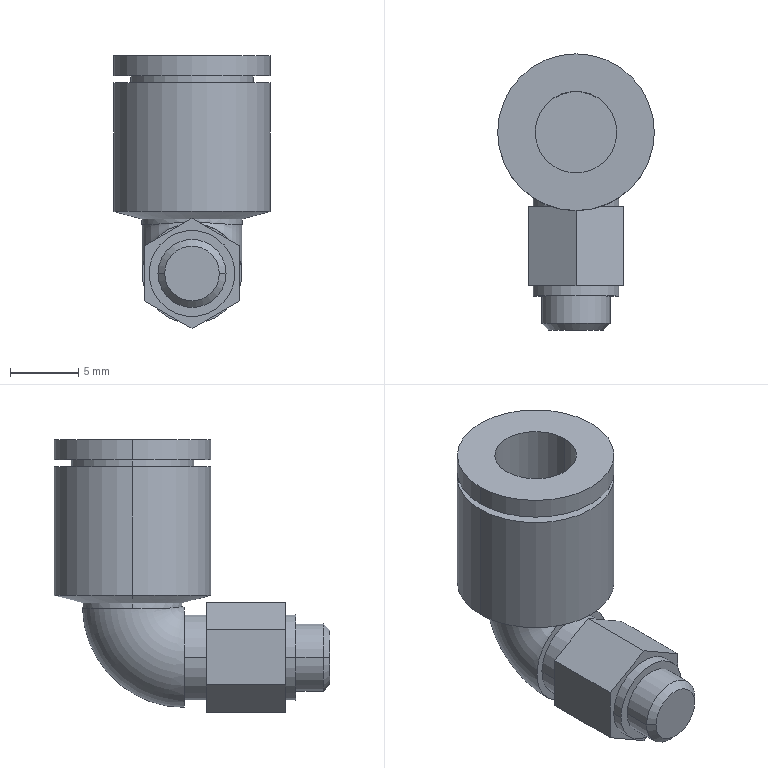Part | SolidWorks | features Revolution 3, ICE 2 | 1 solid | 38 faces | box 11.5 x 20.25 x 20.041 mm | volume 1442 mm3 | cylinder 16 | plane 16 | cone 4 | torus 2 | commonest cylinder face diameters 6.3 x4 11.5 x4 5 x2 6 x2 7.36 x2 9 x2
STEP:
#1=CARTESIAN_POINT('',(0.,18.166,3.565));
#2=VERTEX_POINT('',#1);
#3=CARTESIAN_POINT('',(-2.939,12.285,3.565));
#4=VERTEX_POINT('',#3);
#5=CARTESIAN_POINT('',(0.,18.166,3.565));
#6=CARTESIAN_POINT('',(-0.3422,18.166,3.565));
#7=CARTESIAN_POINT('',(-0.6763,18.119,3.565));
#8=CARTESIAN_POINT('',(-1.166,17.98,3.565));
#9=CARTESIAN_POINT('',(-1.328,17.922,3.565));
#10=CARTESIAN_POINT('',(-1.637,17.785,3.565));
#11=CARTESIAN_POINT('',(-1.787,17.706,3.565));
#12=CARTESIAN_POINT('',(-2.217,17.44,3.565));
#13=CARTESIAN_POINT('',(-2.484,17.219,3.565));
#14=CARTESIAN_POINT('',(-2.825,16.845,3.565));
#15=CARTESIAN_POINT('',(-2.93,16.713,3.565));
#16=CARTESIAN_POINT('',(-3.122,16.432,3.565));
#17=CARTESIAN_POINT('',(-3.209,16.284,3.565));
#18=CARTESIAN_POINT('',(-3.36,15.982,3.565));
#19=CARTESIAN_POINT('',(-3.424,15.826,3.565));
#20=CARTESIAN_POINT('',(-3.532,15.505,3.565));
#21=CARTESIAN_POINT('',(-3.575,15.339,3.565));
#22=CARTESIAN_POINT('',(-3.67,14.838,3.565));
#23=CARTESIAN_POINT('',(-3.686,14.501,3.565));
#24=CARTESIAN_POINT('',(-3.624,13.822,3.565));
#25=CARTESIAN_POINT('',(-3.547,13.491,3.565));
#26=CARTESIAN_POINT('',(-3.366,13.016,3.565));
#27=CARTESIAN_POINT('',(-3.294,12.86,3.565));
#28=CARTESIAN_POINT('',(-3.13,12.563,3.565));
#29=CARTESIAN_POINT('',(-3.039,12.421,3.565));
#30=CARTESIAN_POINT('',(-2.939,12.285,3.565));
#31=B_SPLINE_CURVE_WITH_KNOTS('',3,(#5,#6,#7,#8,#9,#10,#11,#12,#13,#14,#15,#16,#17,#18,#19,#20,#21,#22,#23,#24,#25,#26,#27,#28,#29,#30),.UNSPECIFIED.,.F.,.F.,(4,2,2,2,2,2,2,2,2,2,2,2,4),(0.,0.001012,0.001518,0.002024,0.003036,0.003542,0.004048,0.004554,0.00506,0.006072,0.007083,0.007589,0.008095),.UNSPECIFIED.);
#32=EDGE_CURVE('',#2,#4,#31,.T.);
#33=ORIENTED_EDGE('',*,*,#32,.F.);
#34=CARTESIAN_POINT('',(0.,10.705,-3.67));
#35=VERTEX_POINT('',#34);
#36=CARTESIAN_POINT('',(0.,10.705,3.795));
#37=DIRECTION('',(-1.,0.,0.));
#38=DIRECTION('',(0.,0.,1.));
#39=AXIS2_PLACEMENT_3D('',#36,#37,#38);
#40=CIRCLE('',#39,7.465);
#41=EDGE_CURVE('',#2,#35,#40,.T.);
#42=ORIENTED_EDGE('',*,*,#41,.T.);
#43=CARTESIAN_POINT('',(0.,10.705,3.67));
#44=VERTEX_POINT('',#43);
#45=CARTESIAN_POINT('',(0.,10.705,0.));
#46=DIRECTION('',(0.,1.,0.));
#47=DIRECTION('',(-1.,0.,0.));
#48=AXIS2_PLACEMENT_3D('',#45,#46,#47);
#49=CIRCLE('',#48,3.67);
#50=EDGE_CURVE('',#35,#44,#49,.T.);
#51=ORIENTED_EDGE('',*,*,#50,.T.);
#52=CARTESIAN_POINT('',(0.,10.82,3.746));
#53=VERTEX_POINT('',#52);
#54=CARTESIAN_POINT('',(0.,10.705,3.795));
#55=DIRECTION('',(-1.,0.,0.));
#56=DIRECTION('',(0.,0.,1.));
#57=AXIS2_PLACEMENT_3D('',#54,#55,#56);
#58=CIRCLE('',#57,0.125);
#59=EDGE_CURVE('',#53,#44,#58,.T.);
#60=ORIENTED_EDGE('',*,*,#59,.F.);
#61=CARTESIAN_POINT('',(-2.939,12.285,3.565));
#62=CARTESIAN_POINT('',(-2.767,12.057,3.593));
#63=CARTESIAN_POINT('',(-2.572,11.853,3.616));
#64=CARTESIAN_POINT('',(-2.137,11.491,3.656));
#65=CARTESIAN_POINT('',(-1.895,11.333,3.673));
#66=CARTESIAN_POINT('',(-1.389,11.081,3.704));
#67=CARTESIAN_POINT('',(-1.121,10.983,3.717));
#68=CARTESIAN_POINT('',(-0.5648,10.852,3.739));
#69=CARTESIAN_POINT('',(-0.2838,10.82,3.746));
#70=CARTESIAN_POINT('',(0.,10.82,3.746));
#71=B_SPLINE_CURVE_WITH_KNOTS('',3,(#61,#62,#63,#64,#65,#66,#67,#68,#69,#70),.UNSPECIFIED.,.F.,.F.,(4,2,2,2,4),(0.000001984,0.0008506,0.001699,0.002548,0.003397),.UNSPECIFIED.);
#72=EDGE_CURVE('',#4,#53,#71,.T.);
#73=ORIENTED_EDGE('',*,*,#72,.F.);
#74=EDGE_LOOP('',(#33,#42,#51,#60,#73));
#75=FACE_OUTER_BOUND('',#74,.T.);
#76=CARTESIAN_POINT('',(0.,10.705,3.795));
#77=DIRECTION('',(-1.,0.,0.));
#78=DIRECTION('',(0.,0.,1.));
#79=AXIS2_PLACEMENT_3D('',#76,#77,#78);
#80=TOROIDAL_SURFACE('',#79,3.795,3.67);
#81=ADVANCED_FACE('',(#75),#80,.T.);
#82=CARTESIAN_POINT('',(-3.,14.5,16.));
#83=VERTEX_POINT('',#82);
#84=CARTESIAN_POINT('',(3.,14.5,16.));
#85=VERTEX_POINT('',#84);
#86=CARTESIAN_POINT('',(0.,14.5,16.));
#87=DIRECTION('',(0.,0.,1.));
#88=DIRECTION('',(-1.,0.,0.));
#89=AXIS2_PLACEMENT_3D('',#86,#87,#88);
#90=CIRCLE('',#89,3.);
#91=EDGE_CURVE('',#83,#85,#90,.T.);
#92=ORIENTED_EDGE('',*,*,#91,.T.);
#93=CARTESIAN_POINT('',(3.,14.5,2.));
#94=VERTEX_POINT('',#93);
#95=CARTESIAN_POINT('',(3.,14.5,30.));
#96=DIRECTION('',(0.,0.,-1.));
#97=VECTOR('',#96,1000.);
#98=LINE('',#95,#97);
#99=EDGE_CURVE('',#85,#94,#98,.T.);
#100=ORIENTED_EDGE('',*,*,#99,.T.);
#101=CARTESIAN_POINT('',(-3.,14.5,2.));
#102=VERTEX_POINT('',#101);
#103=CARTESIAN_POINT('',(0.,14.5,2.));
#104=DIRECTION('',(0.,0.,1.));
#105=DIRECTION('',(1.,0.,0.));
#106=AXIS2_PLACEMENT_3D('',#103,#104,#105);
#107=CIRCLE('',#106,3.);
#108=EDGE_CURVE('',#102,#94,#107,.T.);
#109=ORIENTED_EDGE('',*,*,#108,.F.);
#110=CARTESIAN_POINT('',(-3.,14.5,30.));
#111=DIRECTION('',(0.,0.,-1.));
#112=VECTOR('',#111,1000.);
#113=LINE('',#110,#112);
#114=EDGE_CURVE('',#83,#102,#113,.T.);
#115=ORIENTED_EDGE('',*,*,#114,.F.);
#116=EDGE_LOOP('',(#92,#100,#109,#115));
#117=FACE_OUTER_BOUND('',#116,.T.);
#118=CARTESIAN_POINT('',(0.,14.5,30.));
#119=DIRECTION('',(0.,0.,-1.));
#120=DIRECTION('',(-1.,0.,0.));
#121=AXIS2_PLACEMENT_3D('',#118,#119,#120);
#122=CYLINDRICAL_SURFACE('',#121,3.);
#123=ADVANCED_FACE('',(#117),#122,.F.);
#124=CARTESIAN_POINT('',(3.68,14.5,4.));
#125=VERTEX_POINT('',#124);
#126=CARTESIAN_POINT('',(-3.68,14.5,4.));
#127=VERTEX_POINT('',#126);
#128=CARTESIAN_POINT('',(0.,14.5,4.));
#129=DIRECTION('',(0.,0.,1.));
#130=DIRECTION('',(1.,0.,0.));
#131=AXIS2_PLACEMENT_3D('',#128,#129,#130);
#132=CIRCLE('',#131,3.68);
#133=EDGE_CURVE('',#125,#127,#132,.T.);
#134=ORIENTED_EDGE('',*,*,#133,.T.);
#135=CARTESIAN_POINT('',(-5.75,14.5,4.555));
#136=VERTEX_POINT('',#135);
#137=CARTESIAN_POINT('',(-3.68,14.5,4.));
#138=DIRECTION('',(-0.9659,0.,0.2588));
#139=VECTOR('',#138,1000.);
#140=LINE('',#137,#139);
#141=EDGE_CURVE('',#127,#136,#140,.T.);
#142=ORIENTED_EDGE('',*,*,#141,.T.);
#143=CARTESIAN_POINT('',(5.75,14.5,4.555));
#144=VERTEX_POINT('',#143);
#145=CARTESIAN_POINT('',(0.,14.5,4.555));
#146=DIRECTION('',(0.,0.,1.));
#147=DIRECTION('',(1.,0.,0.));
#148=AXIS2_PLACEMENT_3D('',#145,#146,#147);
#149=CIRCLE('',#148,5.75);
#150=EDGE_CURVE('',#144,#136,#149,.T.);
#151=ORIENTED_EDGE('',*,*,#150,.F.);
#152=CARTESIAN_POINT('',(3.68,14.5,4.));
#153=DIRECTION('',(0.9659,0.,0.2588));
#154=VECTOR('',#153,1000.);
#155=LINE('',#152,#154);
#156=EDGE_CURVE('',#125,#144,#155,.T.);
#157=ORIENTED_EDGE('',*,*,#156,.F.);
#158=EDGE_LOOP('',(#134,#142,#151,#157));
#159=FACE_OUTER_BOUND('',#158,.T.);
#160=CARTESIAN_POINT('',(0.,14.5,4.));
#161=DIRECTION('',(0.,0.,1.));
#162=DIRECTION('',(1.,0.,0.));
#163=AXIS2_PLACEMENT_3D('',#160,#161,#162);
#164=CONICAL_SURFACE('',#163,3.68,1.309);
#165=ADVANCED_FACE('',(#159),#164,.T.);
#166=ORIENTED_EDGE('',*,*,#150,.T.);
#167=CARTESIAN_POINT('',(-5.75,14.5,14.));
#168=VERTEX_POINT('',#167);
#169=CARTESIAN_POINT('',(-5.75,14.5,3.565));
#170=DIRECTION('',(0.,0.,1.));
#171=VECTOR('',#170,1000.);
#172=LINE('',#169,#171);
#173=EDGE_CURVE('',#136,#168,#172,.T.);
#174=ORIENTED_EDGE('',*,*,#173,.T.);
#175=CARTESIAN_POINT('',(5.75,14.5,14.));
#176=VERTEX_POINT('',#175);
#177=CARTESIAN_POINT('',(0.,14.5,14.));
#178=DIRECTION('',(0.,0.,1.));
#179=DIRECTION('',(1.,0.,0.));
#180=AXIS2_PLACEMENT_3D('',#177,#178,#179);
#181=CIRCLE('',#180,5.75);
#182=EDGE_CURVE('',#176,#168,#181,.T.);
#183=ORIENTED_EDGE('',*,*,#182,.F.);
#184=CARTESIAN_POINT('',(5.75,14.5,3.565));
#185=DIRECTION('',(0.,0.,1.));
#186=VECTOR('',#185,1000.);
#187=LINE('',#184,#186);
#188=EDGE_CURVE('',#144,#176,#187,.T.);
#189=ORIENTED_EDGE('',*,*,#188,.F.);
#190=EDGE_LOOP('',(#166,#174,#183,#189));
#191=FACE_OUTER_BOUND('',#190,.T.);
#192=CARTESIAN_POINT('',(0.,14.5,3.565));
#193=DIRECTION('',(0.,0.,1.));
#194=DIRECTION('',(1.,0.,0.));
#195=AXIS2_PLACEMENT_3D('',#192,#193,#194);
#196=CYLINDRICAL_SURFACE('',#195,5.75);
#197=ADVANCED_FACE('',(#191),#196,.T.);
#198=CARTESIAN_POINT('',(4.5,14.5,14.));
#199=VERTEX_POINT('',#198);
#200=CARTESIAN_POINT('',(-4.5,14.5,14.));
#201=VERTEX_POINT('',#200);
#202=CARTESIAN_POINT('',(0.,14.5,14.));
#203=DIRECTION('',(0.,0.,1.));
#204=DIRECTION('',(1.,0.,0.));
#205=AXIS2_PLACEMENT_3D('',#202,#203,#204);
#206=CIRCLE('',#205,4.5);
#207=EDGE_CURVE('',#199,#201,#206,.T.);
#208=ORIENTED_EDGE('',*,*,#207,.T.);
#209=CARTESIAN_POINT('',(-4.5,14.5,14.5));
#210=VERTEX_POINT('',#209);
#211=CARTESIAN_POINT('',(-4.5,14.5,3.565));
#212=DIRECTION('',(0.,0.,1.));
#213=VECTOR('',#212,1000.);
#214=LINE('',#211,#213);
#215=EDGE_CURVE('',#201,#210,#214,.T.);
#216=ORIENTED_EDGE('',*,*,#215,.T.);
#217=CARTESIAN_POINT('',(4.5,14.5,14.5));
#218=VERTEX_POINT('',#217);
#219=CARTESIAN_POINT('',(0.,14.5,14.5));
#220=DIRECTION('',(0.,0.,1.));
#221=DIRECTION('',(1.,0.,0.));
#222=AXIS2_PLACEMENT_3D('',#219,#220,#221);
#223=CIRCLE('',#222,4.5);
#224=EDGE_CURVE('',#218,#210,#223,.T.);
#225=ORIENTED_EDGE('',*,*,#224,.F.);
#226=CARTESIAN_POINT('',(4.5,14.5,3.565));
#227=DIRECTION('',(0.,0.,1.));
#228=VECTOR('',#227,1000.);
#229=LINE('',#226,#228);
#230=EDGE_CURVE('',#199,#218,#229,.T.);
#231=ORIENTED_EDGE('',*,*,#230,.F.);
#232=EDGE_LOOP('',(#208,#216,#225,#231));
#233=FACE_OUTER_BOUND('',#232,.T.);
#234=CARTESIAN_POINT('',(0.,14.5,3.565));
#235=DIRECTION('',(0.,0.,1.));
#236=DIRECTION('',(1.,0.,0.));
#237=AXIS2_PLACEMENT_3D('',#234,#235,#236);
#238=CYLINDRICAL_SURFACE('',#237,4.5);
#239=ADVANCED_FACE('',(#233),#238,.T.);
#240=CARTESIAN_POINT('',(5.75,14.5,14.5));
#241=VERTEX_POINT('',#240);
#242=CARTESIAN_POINT('',(-5.75,14.5,14.5));
#243=VERTEX_POINT('',#242);
#244=CARTESIAN_POINT('',(0.,14.5,14.5));
#245=DIRECTION('',(0.,0.,1.));
#246=DIRECTION('',(1.,0.,0.));
#247=AXIS2_PLACEMENT_3D('',#244,#245,#246);
#248=CIRCLE('',#247,5.75);
#249=EDGE_CURVE('',#241,#243,#248,.T.);
#250=ORIENTED_EDGE('',*,*,#249,.T.);
#251=CARTESIAN_POINT('',(-5.75,14.5,16.));
#252=VERTEX_POINT('',#251);
#253=CARTESIAN_POINT('',(-5.75,14.5,3.565));
#254=DIRECTION('',(0.,0.,1.));
#255=VECTOR('',#254,1000.);
#256=LINE('',#253,#255);
#257=EDGE_CURVE('',#243,#252,#256,.T.);
#258=ORIENTED_EDGE('',*,*,#257,.T.);
#259=CARTESIAN_POINT('',(5.75,14.5,16.));
#260=VERTEX_POINT('',#259);
#261=CARTESIAN_POINT('',(0.,14.5,16.));
#262=DIRECTION('',(0.,0.,1.));
#263=DIRECTION('',(1.,0.,0.));
#264=AXIS2_PLACEMENT_3D('',#261,#262,#263);
#265=CIRCLE('',#264,5.75);
#266=EDGE_CURVE('',#260,#252,#265,.T.);
#267=ORIENTED_EDGE('',*,*,#266,.F.);
#268=CARTESIAN_POINT('',(5.75,14.5,3.565));
#269=DIRECTION('',(0.,0.,1.));
#270=VECTOR('',#269,1000.);
#271=LINE('',#268,#270);
#272=EDGE_CURVE('',#241,#260,#271,.T.);
#273=ORIENTED_EDGE('',*,*,#272,.F.);
#274=EDGE_LOOP('',(#250,#258,#267,#273));
#275=FACE_OUTER_BOUND('',#274,.T.);
#276=CARTESIAN_POINT('',(0.,14.5,3.565));
#277=DIRECTION('',(0.,0.,1.));
#278=DIRECTION('',(1.,0.,0.));
#279=AXIS2_PLACEMENT_3D('',#276,#277,#278);
#280=CYLINDRICAL_SURFACE('',#279,5.75);
#281=ADVANCED_FACE('',(#275),#280,.T.);
#282=CARTESIAN_POINT('',(3.68,14.5,3.565));
#283=VERTEX_POINT('',#282);
#284=CARTESIAN_POINT('',(-3.68,14.5,3.565));
#285=VERTEX_POINT('',#284);
#286=CARTESIAN_POINT('',(0.,14.5,3.565));
#287=DIRECTION('',(0.,0.,1.));
#288=DIRECTION('',(1.,0.,0.));
#289=AXIS2_PLACEMENT_3D('',#286,#287,#288);
#290=CIRCLE('',#289,3.68);
#291=EDGE_CURVE('',#283,#285,#290,.T.);
#292=ORIENTED_EDGE('',*,*,#291,.T.);
#293=CARTESIAN_POINT('',(-3.68,14.5,3.565));
#294=DIRECTION('',(0.,0.,1.));
#295=VECTOR('',#294,1000.);
#296=LINE('',#293,#295);
#297=EDGE_CURVE('',#285,#127,#296,.T.);
#298=ORIENTED_EDGE('',*,*,#297,.T.);
#299=ORIENTED_EDGE('',*,*,#133,.F.);
#300=CARTESIAN_POINT('',(3.68,14.5,3.565));
#301=DIRECTION('',(0.,0.,1.));
#302=VECTOR('',#301,1000.);
#303=LINE('',#300,#302);
#304=EDGE_CURVE('',#283,#125,#303,.T.);
#305=ORIENTED_EDGE('',*,*,#304,.F.);
#306=EDGE_LOOP('',(#292,#298,#299,#305));
#307=FACE_OUTER_BOUND('',#306,.T.);
#308=CARTESIAN_POINT('',(0.,14.5,3.565));
#309=DIRECTION('',(0.,0.,1.));
#310=DIRECTION('',(1.,0.,0.));
#311=AXIS2_PLACEMENT_3D('',#308,#309,#310);
#312=CYLINDRICAL_SURFACE('',#311,3.68);
#313=ADVANCED_FACE('',(#307),#312,.T.);
#314=CARTESIAN_POINT('',(-3.15,10.705,0.));
#315=VERTEX_POINT('',#314);
#316=CARTESIAN_POINT('',(3.15,10.705,0.));
#317=VERTEX_POINT('',#316);
#318=CARTESIAN_POINT('',(0.,10.705,0.));
#319=DIRECTION('',(0.,1.,0.));
#320=DIRECTION('',(-1.,0.,0.));
#321=AXIS2_PLACEMENT_3D('',#318,#319,#320);
#322=CIRCLE('',#321,3.15);
#323=EDGE_CURVE('',#315,#317,#322,.T.);
#324=ORIENTED_EDGE('',*,*,#323,.F.);
#325=CARTESIAN_POINT('',(-3.15,9.05,0.));
#326=VERTEX_POINT('',#325);
#327=CARTESIAN_POINT('',(-3.15,10.705,0.));
#328=DIRECTION('',(0.,-1.,0.));
#329=VECTOR('',#328,1000.);
#330=LINE('',#327,#329);
#331=EDGE_CURVE('',#315,#326,#330,.T.);
#332=ORIENTED_EDGE('',*,*,#331,.T.);
#333=CARTESIAN_POINT('',(3.15,9.05,0.));
#334=VERTEX_POINT('',#333);
#335=CARTESIAN_POINT('',(0.,9.05,0.));
#336=DIRECTION('',(0.,1.,0.));
#337=DIRECTION('',(0.,0.,1.));
#338=AXIS2_PLACEMENT_3D('',#335,#336,#337);
#339=CIRCLE('',#338,3.15);
#340=EDGE_CURVE('',#326,#334,#339,.T.);
#341=ORIENTED_EDGE('',*,*,#340,.T.);
#342=CARTESIAN_POINT('',(3.15,10.705,0.));
#343=DIRECTION('',(0.,-1.,0.));
#344=VECTOR('',#343,1000.);
#345=LINE('',#342,#344);
#346=EDGE_CURVE('',#317,#334,#345,.T.);
#347=ORIENTED_EDGE('',*,*,#346,.F.);
#348=EDGE_LOOP('',(#324,#332,#341,#347));
#349=FACE_OUTER_BOUND('',#348,.T.);
#350=CARTESIAN_POINT('',(0.,10.705,0.));
#351=DIRECTION('',(0.,-1.,0.));
#352=DIRECTION('',(1.,0.,0.));
#353=AXIS2_PLACEMENT_3D('',#350,#351,#352);
#354=CYLINDRICAL_SURFACE('',#353,3.15);
#355=ADVANCED_FACE('',(#349),#354,.T.);
#356=CARTESIAN_POINT('',(2.5,2.5,0.));
#357=VERTEX_POINT('',#356);
#358=CARTESIAN_POINT('',(-2.5,2.5,0.));
#359=VERTEX_POINT('',#358);
#360=CARTESIAN_POINT('',(0.,2.5,0.));
#361=DIRECTION('',(0.,-1.,0.));
#362=DIRECTION('',(1.,0.,0.));
#363=AXIS2_PLACEMENT_3D('',#360,#361,#362);
#364=CIRCLE('',#363,2.5);
#365=EDGE_CURVE('',#357,#359,#364,.T.);
#366=ORIENTED_EDGE('',*,*,#365,.T.);
#367=CARTESIAN_POINT('',(-2.5,0.49,0.));
#368=VERTEX_POINT('',#367);
#369=CARTESIAN_POINT('',(-2.5,10.705,0.));
#370=DIRECTION('',(0.,-1.,0.));
#371=VECTOR('',#370,1000.);
#372=LINE('',#369,#371);
#373=EDGE_CURVE('',#359,#368,#372,.T.);
#374=ORIENTED_EDGE('',*,*,#373,.T.);
#375=CARTESIAN_POINT('',(2.5,0.49,0.));
#376=VERTEX_POINT('',#375);
#377=CARTESIAN_POINT('',(0.,0.49,0.));
#378=DIRECTION('',(0.,-1.,0.));
#379=DIRECTION('',(1.,0.,0.));
#380=AXIS2_PLACEMENT_3D('',#377,#378,#379);
#381=CIRCLE('',#380,2.5);
#382=EDGE_CURVE('',#376,#368,#381,.T.);
#383=ORIENTED_EDGE('',*,*,#382,.F.);
#384=CARTESIAN_POINT('',(2.5,10.705,0.));
#385=DIRECTION('',(0.,-1.,0.));
#386=VECTOR('',#385,1000.);
#387=LINE('',#384,#386);
#388=EDGE_CURVE('',#357,#376,#387,.T.);
#389=ORIENTED_EDGE('',*,*,#388,.F.);
#390=EDGE_LOOP('',(#366,#374,#383,#389));
#391=FACE_OUTER_BOUND('',#390,.T.);
#392=CARTESIAN_POINT('',(0.,10.705,0.));
#393=DIRECTION('',(0.,-1.,0.));
#394=DIRECTION('',(1.,0.,0.));
#395=AXIS2_PLACEMENT_3D('',#392,#393,#394);
#396=CYLINDRICAL_SURFACE('',#395,2.5);
#397=ADVANCED_FACE('',(#391),#396,.T.);
#398=CARTESIAN_POINT('',(2.01,0.,0.));
#399=VERTEX_POINT('',#398);
#400=CARTESIAN_POINT('',(-2.01,0.,0.));
#401=VERTEX_POINT('',#400);
#402=CARTESIAN_POINT('',(0.,0.,0.));
#403=DIRECTION('',(0.,-1.,0.));
#404=DIRECTION('',(1.,0.,0.));
#405=AXIS2_PLACEMENT_3D('',#402,#403,#404);
#406=CIRCLE('',#405,2.01);
#407=EDGE_CURVE('',#399,#401,#406,.T.);
#408=ORIENTED_EDGE('',*,*,#407,.F.);
#409=CARTESIAN_POINT('',(2.5,0.49,0.));
#410=DIRECTION('',(0.7071,0.7071,0.));
#411=VECTOR('',#410,1000.);
#412=LINE('',#409,#411);
#413=EDGE_CURVE('',#399,#376,#412,.T.);
#414=ORIENTED_EDGE('',*,*,#413,.T.);
#415=ORIENTED_EDGE('',*,*,#382,.T.);
#416=CARTESIAN_POINT('',(-2.5,0.49,0.));
#417=DIRECTION('',(-0.7071,0.7071,0.));
#418=VECTOR('',#417,1000.);
#419=LINE('',#416,#418);
#420=EDGE_CURVE('',#401,#368,#419,.T.);
#421=ORIENTED_EDGE('',*,*,#420,.F.);
#422=EDGE_LOOP('',(#408,#414,#415,#421));
#423=FACE_OUTER_BOUND('',#422,.T.);
#424=CARTESIAN_POINT('',(0.,0.49,0.));
#425=DIRECTION('',(0.,1.,0.));
#426=DIRECTION('',(-1.,0.,0.));
#427=AXIS2_PLACEMENT_3D('',#424,#425,#426);
#428=CONICAL_SURFACE('',#427,2.5,0.7854);
#429=ADVANCED_FACE('',(#423),#428,.T.);
#430=CARTESIAN_POINT('',(-3.15,3.25,0.));
#431=VERTEX_POINT('',#430);
#432=CARTESIAN_POINT('',(3.15,3.25,0.));
#433=VERTEX_POINT('',#432);
#434=CARTESIAN_POINT('',(0.,3.25,0.));
#435=DIRECTION('',(0.,1.,0.));
#436=DIRECTION('',(0.,0.,1.));
#437=AXIS2_PLACEMENT_3D('',#434,#435,#436);
#438=CIRCLE('',#437,3.15);
#439=EDGE_CURVE('',#431,#433,#438,.T.);
#440=ORIENTED_EDGE('',*,*,#439,.F.);
#441=CARTESIAN_POINT('',(-3.15,2.5,0.));
#442=VERTEX_POINT('',#441);
#443=CARTESIAN_POINT('',(-3.15,10.705,0.));
#444=DIRECTION('',(0.,-1.,0.));
#445=VECTOR('',#444,1000.);
#446=LINE('',#443,#445);
#447=EDGE_CURVE('',#431,#442,#446,.T.);
#448=ORIENTED_EDGE('',*,*,#447,.T.);
#449=CARTESIAN_POINT('',(3.15,2.5,0.));
#450=VERTEX_POINT('',#449);
#451=CARTESIAN_POINT('',(0.,2.5,0.));
#452=DIRECTION('',(0.,-1.,0.));
#453=DIRECTION('',(1.,0.,0.));
#454=AXIS2_PLACEMENT_3D('',#451,#452,#453);
#455=CIRCLE('',#454,3.15);
#456=EDGE_CURVE('',#450,#442,#455,.T.);
#457=ORIENTED_EDGE('',*,*,#456,.F.);
#458=CARTESIAN_POINT('',(3.15,10.705,0.));
#459=DIRECTION('',(0.,-1.,0.));
#460=VECTOR('',#459,1000.);
#461=LINE('',#458,#460);
#462=EDGE_CURVE('',#433,#450,#461,.T.);
#463=ORIENTED_EDGE('',*,*,#462,.F.);
#464=EDGE_LOOP('',(#440,#448,#457,#463));
#465=FACE_OUTER_BOUND('',#464,.T.);
#466=CARTESIAN_POINT('',(0.,10.705,0.));
#467=DIRECTION('',(0.,-1.,0.));
#468=DIRECTION('',(1.,0.,0.));
#469=AXIS2_PLACEMENT_3D('',#466,#467,#468);
#470=CYLINDRICAL_SURFACE('',#469,3.15);
#471=ADVANCED_FACE('',(#465),#470,.T.);
#472=ORIENTED_EDGE('',*,*,#266,.T.);
#473=CARTESIAN_POINT('',(0.,14.5,16.));
#474=DIRECTION('',(0.,0.,1.));
#475=DIRECTION('',(1.,0.,0.));
#476=AXIS2_PLACEMENT_3D('',#473,#474,#475);
#477=CIRCLE('',#476,5.75);
#478=EDGE_CURVE('',#252,#260,#477,.T.);
#479=ORIENTED_EDGE('',*,*,#478,.T.);
#480=EDGE_LOOP('',(#472,#479));
#481=FACE_OUTER_BOUND('',#480,.T.);
#482=ORIENTED_EDGE('',*,*,#91,.F.);
#483=CARTESIAN_POINT('',(0.,14.5,16.));
#484=DIRECTION('',(0.,0.,1.));
#485=DIRECTION('',(-1.,0.,0.));
#486=AXIS2_PLACEMENT_3D('',#483,#484,#485);
#487=CIRCLE('',#486,3.);
#488=EDGE_CURVE('',#85,#83,#487,.T.);
#489=ORIENTED_EDGE('',*,*,#488,.F.);
#490=EDGE_LOOP('',(#482,#489));
#491=FACE_BOUND('',#490,.T.);
#492=CARTESIAN_POINT('',(0.,14.5,16.));
#493=DIRECTION('',(0.,0.,-1.));
#494=DIRECTION('',(-1.,0.,0.));
#495=AXIS2_PLACEMENT_3D('',#492,#493,#494);
#496=PLANE('',#495);
#497=ADVANCED_FACE('',(#481,#491),#496,.F.);
#498=ORIENTED_EDGE('',*,*,#41,.F.);
#499=CARTESIAN_POINT('',(2.939,12.285,3.565));
#500=VERTEX_POINT('',#499);
#501=CARTESIAN_POINT('',(2.939,12.285,3.565));
#502=CARTESIAN_POINT('',(3.04,12.422,3.565));
#503=CARTESIAN_POINT('',(3.132,12.566,3.565));
#504=CARTESIAN_POINT('',(3.294,12.862,3.565));
#505=CARTESIAN_POINT('',(3.365,13.014,3.565));
#506=CARTESIAN_POINT('',(3.486,13.329,3.565));
#507=CARTESIAN_POINT('',(3.536,13.493,3.565));
#508=CARTESIAN_POINT('',(3.613,13.825,3.565));
#509=CARTESIAN_POINT('',(3.666,14.158,3.565));
#510=CARTESIAN_POINT('',(3.674,14.496,3.565));
#511=CARTESIAN_POINT('',(3.658,14.836,3.565));
#512=CARTESIAN_POINT('',(3.638,15.006,3.565));
#513=CARTESIAN_POINT('',(3.576,15.338,3.565));
#514=CARTESIAN_POINT('',(3.533,15.501,3.565));
#515=CARTESIAN_POINT('',(3.426,15.822,3.565));
#516=CARTESIAN_POINT('',(3.36,15.98,3.565));
#517=CARTESIAN_POINT('',(3.133,16.437,3.565));
#518=CARTESIAN_POINT('',(2.943,16.715,3.565));
#519=CARTESIAN_POINT('',(2.484,17.219,3.565));
#520=CARTESIAN_POINT('',(2.222,17.436,3.565));
#521=CARTESIAN_POINT('',(1.791,17.704,3.565));
#522=CARTESIAN_POINT('',(1.639,17.784,3.565));
#523=CARTESIAN_POINT('',(1.328,17.922,3.565));
#524=CARTESIAN_POINT('',(1.17,17.979,3.565));
#525=CARTESIAN_POINT('',(0.8455,18.072,3.565));
#526=CARTESIAN_POINT('',(0.6799,18.107,3.565));
#527=CARTESIAN_POINT('',(0.4261,18.143,3.565));
#528=CARTESIAN_POINT('',(0.341,18.152,3.565));
#529=CARTESIAN_POINT('',(0.1708,18.163,3.565));
#530=CARTESIAN_POINT('',(0.08395,18.166,3.565));
#531=CARTESIAN_POINT('',(0.,18.166,3.565));
#532=B_SPLINE_CURVE_WITH_KNOTS('',3,(#501,#502,#503,#504,#505,#506,#507,#508,#509,#510,#511,#512,#513,#514,#515,#516,#517,#518,#519,#520,#521,#522,#523,#524,#525,#526,#527,#528,#529,#530,#531),.UNSPECIFIED.,.F.,.F.,(4,2,2,2,1,2,2,2,2,2,2,2,2,2,2,4),(0.03478,0.03528,0.03578,0.03627,0.03677,0.03727,0.03776,0.03826,0.03876,0.03975,0.04074,0.04124,0.04174,0.04223,0.04248,0.04273),.UNSPECIFIED.);
#533=EDGE_CURVE('',#500,#2,#532,.T.);
#534=ORIENTED_EDGE('',*,*,#533,.F.);
#535=CARTESIAN_POINT('',(0.,10.82,3.746));
#536=CARTESIAN_POINT('',(0.2832,10.82,3.746));
#537=CARTESIAN_POINT('',(0.5699,10.853,3.739));
#538=CARTESIAN_POINT('',(1.119,10.983,3.717));
#539=CARTESIAN_POINT('',(1.389,11.08,3.704));
#540=CARTESIAN_POINT('',(1.897,11.334,3.673));
#541=CARTESIAN_POINT('',(2.133,11.488,3.656));
#542=CARTESIAN_POINT('',(2.569,11.85,3.616));
#543=CARTESIAN_POINT('',(2.767,12.057,3.593));
#544=CARTESIAN_POINT('',(2.939,12.285,3.565));
#545=B_SPLINE_CURVE_WITH_KNOTS('',3,(#535,#536,#537,#538,#539,#540,#541,#542,#543,#544),.UNSPECIFIED.,.F.,.F.,(4,2,2,2,4),(0.003397,0.004243,0.00509,0.005937,0.006784),.UNSPECIFIED.);
#546=EDGE_CURVE('',#53,#500,#545,.T.);
#547=ORIENTED_EDGE('',*,*,#546,.F.);
#548=ORIENTED_EDGE('',*,*,#59,.T.);
#549=CARTESIAN_POINT('',(0.,10.705,0.));
#550=DIRECTION('',(0.,1.,0.));
#551=DIRECTION('',(-1.,0.,0.));
#552=AXIS2_PLACEMENT_3D('',#549,#550,#551);
#553=CIRCLE('',#552,3.67);
#554=EDGE_CURVE('',#44,#35,#553,.T.);
#555=ORIENTED_EDGE('',*,*,#554,.T.);
#556=EDGE_LOOP('',(#498,#534,#547,#548,#555));
#557=FACE_OUTER_BOUND('',#556,.T.);
#558=CARTESIAN_POINT('',(0.,10.705,3.795));
#559=DIRECTION('',(-1.,0.,0.));
#560=DIRECTION('',(0.,0.,1.));
#561=AXIS2_PLACEMENT_3D('',#558,#559,#560);
#562=TOROIDAL_SURFACE('',#561,3.795,3.67);
#563=ADVANCED_FACE('',(#557),#562,.T.);
#564=ORIENTED_EDGE('',*,*,#447,.F.);
#565=CARTESIAN_POINT('',(0.,3.25,0.));
#566=DIRECTION('',(0.,1.,0.));
#567=DIRECTION('',(0.,0.,1.));
#568=AXIS2_PLACEMENT_3D('',#565,#566,#567);
#569=CIRCLE('',#568,3.15);
#570=EDGE_CURVE('',#433,#431,#569,.T.);
#571=ORIENTED_EDGE('',*,*,#570,.F.);
#572=ORIENTED_EDGE('',*,*,#462,.T.);
#573=CARTESIAN_POINT('',(0.,2.5,0.));
#574=DIRECTION('',(0.,-1.,0.));
#575=DIRECTION('',(1.,0.,0.));
#576=AXIS2_PLACEMENT_3D('',#573,#574,#575);
#577=CIRCLE('',#576,3.15);
#578=EDGE_CURVE('',#442,#450,#577,.T.);
#579=ORIENTED_EDGE('',*,*,#578,.F.);
#580=EDGE_LOOP('',(#564,#571,#572,#579));
#581=FACE_OUTER_BOUND('',#580,.T.);
#582=CARTESIAN_POINT('',(0.,10.705,0.));
#583=DIRECTION('',(0.,-1.,0.));
#584=DIRECTION('',(1.,0.,0.));
#585=AXIS2_PLACEMENT_3D('',#582,#583,#584);
#586=CYLINDRICAL_SURFACE('',#585,3.15);
#587=ADVANCED_FACE('',(#581),#586,.T.);
#588=CARTESIAN_POINT('',(0.,0.,0.));
#589=DIRECTION('',(0.,-1.,0.));
#590=DIRECTION('',(1.,0.,0.));
#591=AXIS2_PLACEMENT_3D('',#588,#589,#590);
#592=CIRCLE('',#591,2.01);
#593=EDGE_CURVE('',#401,#399,#592,.T.);
#594=ORIENTED_EDGE('',*,*,#593,.T.);
#595=ORIENTED_EDGE('',*,*,#407,.T.);
#596=EDGE_LOOP('',(#594,#595));
#597=FACE_OUTER_BOUND('',#596,.T.);
#598=CARTESIAN_POINT('',(0.,0.,0.));
#599=DIRECTION('',(0.,1.,0.));
#600=DIRECTION('',(-1.,0.,0.));
#601=AXIS2_PLACEMENT_3D('',#598,#599,#600);
#602=PLANE('',#601);
#603=ADVANCED_FACE('',(#597),#602,.F.);
#604=ORIENTED_EDGE('',*,*,#413,.F.);
#605=ORIENTED_EDGE('',*,*,#593,.F.);
#606=ORIENTED_EDGE('',*,*,#420,.T.);
#607=CARTESIAN_POINT('',(0.,0.49,0.));
#608=DIRECTION('',(0.,-1.,0.));
#609=DIRECTION('',(1.,0.,0.));
#610=AXIS2_PLACEMENT_3D('',#607,#608,#609);
#611=CIRCLE('',#610,2.5);
#612=EDGE_CURVE('',#368,#376,#611,.T.);
#613=ORIENTED_EDGE('',*,*,#612,.T.);
#614=EDGE_LOOP('',(#604,#605,#606,#613));
#615=FACE_OUTER_BOUND('',#614,.T.);
#616=CARTESIAN_POINT('',(0.,0.49,0.));
#617=DIRECTION('',(0.,1.,0.));
#618=DIRECTION('',(-1.,0.,0.));
#619=AXIS2_PLACEMENT_3D('',#616,#617,#618);
#620=CONICAL_SURFACE('',#619,2.5,0.7854);
#621=ADVANCED_FACE('',(#615),#620,.T.);
#622=ORIENTED_EDGE('',*,*,#373,.F.);
#623=CARTESIAN_POINT('',(0.,2.5,0.));
#624=DIRECTION('',(0.,-1.,0.));
#625=DIRECTION('',(1.,0.,0.));
#626=AXIS2_PLACEMENT_3D('',#623,#624,#625);
#627=CIRCLE('',#626,2.5);
#628=EDGE_CURVE('',#359,#357,#627,.T.);
#629=ORIENTED_EDGE('',*,*,#628,.T.);
#630=ORIENTED_EDGE('',*,*,#388,.T.);
#631=ORIENTED_EDGE('',*,*,#612,.F.);
#632=EDGE_LOOP('',(#622,#629,#630,#631));
#633=FACE_OUTER_BOUND('',#632,.T.);
#634=CARTESIAN_POINT('',(0.,10.705,0.));
#635=DIRECTION('',(0.,-1.,0.));
#636=DIRECTION('',(1.,0.,0.));
#637=AXIS2_PLACEMENT_3D('',#634,#635,#636);
#638=CYLINDRICAL_SURFACE('',#637,2.5);
#639=ADVANCED_FACE('',(#633),#638,.T.);
#640=ORIENTED_EDGE('',*,*,#365,.F.);
#641=ORIENTED_EDGE('',*,*,#628,.F.);
#642=EDGE_LOOP('',(#640,#641));
#643=FACE_BOUND('',#642,.T.);
#644=ORIENTED_EDGE('',*,*,#456,.T.);
#645=ORIENTED_EDGE('',*,*,#578,.T.);
#646=EDGE_LOOP('',(#644,#645));
#647=FACE_OUTER_BOUND('',#646,.T.);
#648=CARTESIAN_POINT('',(-2.5,2.5,0.));
#649=DIRECTION('',(0.,1.,0.));
#650=DIRECTION('',(-1.,0.,0.));
#651=AXIS2_PLACEMENT_3D('',#648,#649,#650);
#652=PLANE('',#651);
#653=ADVANCED_FACE('',(#643,#647),#652,.F.);
#654=CARTESIAN_POINT('',(0.,9.05,-4.041));
#655=VERTEX_POINT('',#654);
#656=CARTESIAN_POINT('',(-3.5,9.05,-2.021));
#657=VERTEX_POINT('',#656);
#658=CARTESIAN_POINT('',(0.,9.05,-4.041));
#659=DIRECTION('',(-0.866,0.,0.5));
#660=VECTOR('',#659,1000.);
#661=LINE('',#658,#660);
#662=EDGE_CURVE('',#655,#657,#661,.T.);
#663=ORIENTED_EDGE('',*,*,#662,.T.);
#664=CARTESIAN_POINT('',(-3.5,9.05,2.021));
#665=VERTEX_POINT('',#664);
#666=CARTESIAN_POINT('',(-3.5,9.05,-2.021));
#667=DIRECTION('',(0.,0.,1.));
#668=VECTOR('',#667,1000.);
#669=LINE('',#666,#668);
#670=EDGE_CURVE('',#657,#665,#669,.T.);
#671=ORIENTED_EDGE('',*,*,#670,.T.);
#672=CARTESIAN_POINT('',(0.,9.05,4.041));
#673=VERTEX_POINT('',#672);
#674=CARTESIAN_POINT('',(-3.5,9.05,2.021));
#675=DIRECTION('',(0.866,0.,0.5));
#676=VECTOR('',#675,1000.);
#677=LINE('',#674,#676);
#678=EDGE_CURVE('',#665,#673,#677,.T.);
#679=ORIENTED_EDGE('',*,*,#678,.T.);
#680=CARTESIAN_POINT('',(3.5,9.05,2.021));
#681=VERTEX_POINT('',#680);
#682=CARTESIAN_POINT('',(0.,9.05,4.041));
#683=DIRECTION('',(0.866,0.,-0.5));
#684=VECTOR('',#683,1000.);
#685=LINE('',#682,#684);
#686=EDGE_CURVE('',#673,#681,#685,.T.);
#687=ORIENTED_EDGE('',*,*,#686,.T.);
#688=CARTESIAN_POINT('',(3.5,9.05,-2.021));
#689=VERTEX_POINT('',#688);
#690=CARTESIAN_POINT('',(3.5,9.05,2.021));
#691=DIRECTION('',(0.,0.,-1.));
#692=VECTOR('',#691,1000.);
#693=LINE('',#690,#692);
#694=EDGE_CURVE('',#681,#689,#693,.T.);
#695=ORIENTED_EDGE('',*,*,#694,.T.);
#696=CARTESIAN_POINT('',(3.5,9.05,-2.021));
#697=DIRECTION('',(-0.866,0.,-0.5));
#698=VECTOR('',#697,1000.);
#699=LINE('',#696,#698);
#700=EDGE_CURVE('',#689,#655,#699,.T.);
#701=ORIENTED_EDGE('',*,*,#700,.T.);
#702=EDGE_LOOP('',(#663,#671,#679,#687,#695,#701));
#703=FACE_OUTER_BOUND('',#702,.T.);
#704=CARTESIAN_POINT('',(0.,9.05,0.));
#705=DIRECTION('',(0.,1.,0.));
#706=DIRECTION('',(0.,0.,1.));
#707=AXIS2_PLACEMENT_3D('',#704,#705,#706);
#708=CIRCLE('',#707,3.15);
#709=EDGE_CURVE('',#334,#326,#708,.T.);
#710=ORIENTED_EDGE('',*,*,#709,.F.);
#711=ORIENTED_EDGE('',*,*,#340,.F.);
#712=EDGE_LOOP('',(#710,#711));
#713=FACE_BOUND('',#712,.T.);
#714=CARTESIAN_POINT('',(0.,9.05,0.));
#715=DIRECTION('',(0.,1.,0.));
#716=DIRECTION('',(0.,0.,1.));
#717=AXIS2_PLACEMENT_3D('',#714,#715,#716);
#718=PLANE('',#717);
#719=ADVANCED_FACE('',(#703,#713),#718,.T.);
#720=CARTESIAN_POINT('',(0.,3.25,-4.041));
#721=VERTEX_POINT('',#720);
#722=CARTESIAN_POINT('',(-3.5,3.25,-2.021));
#723=VERTEX_POINT('',#722);
#724=CARTESIAN_POINT('',(0.,3.25,-4.041));
#725=DIRECTION('',(-0.866,0.,0.5));
#726=VECTOR('',#725,1000.);
#727=LINE('',#724,#726);
#728=EDGE_CURVE('',#721,#723,#727,.T.);
#729=ORIENTED_EDGE('',*,*,#728,.F.);
#730=CARTESIAN_POINT('',(3.5,3.25,-2.021));
#731=VERTEX_POINT('',#730);
#732=CARTESIAN_POINT('',(3.5,3.25,-2.021));
#733=DIRECTION('',(-0.866,0.,-0.5));
#734=VECTOR('',#733,1000.);
#735=LINE('',#732,#734);
#736=EDGE_CURVE('',#731,#721,#735,.T.);
#737=ORIENTED_EDGE('',*,*,#736,.F.);
#738=CARTESIAN_POINT('',(3.5,3.25,2.021));
#739=VERTEX_POINT('',#738);
#740=CARTESIAN_POINT('',(3.5,3.25,2.021));
#741=DIRECTION('',(0.,0.,-1.));
#742=VECTOR('',#741,1000.);
#743=LINE('',#740,#742);
#744=EDGE_CURVE('',#739,#731,#743,.T.);
#745=ORIENTED_EDGE('',*,*,#744,.F.);
#746=CARTESIAN_POINT('',(0.,3.25,4.041));
#747=VERTEX_POINT('',#746);
#748=CARTESIAN_POINT('',(0.,3.25,4.041));
#749=DIRECTION('',(0.866,0.,-0.5));
#750=VECTOR('',#749,1000.);
#751=LINE('',#748,#750);
#752=EDGE_CURVE('',#747,#739,#751,.T.);
#753=ORIENTED_EDGE('',*,*,#752,.F.);
#754=CARTESIAN_POINT('',(-3.5,3.25,2.021));
#755=VERTEX_POINT('',#754);
#756=CARTESIAN_POINT('',(-3.5,3.25,2.021));
#757=DIRECTION('',(0.866,0.,0.5));
#758=VECTOR('',#757,1000.);
#759=LINE('',#756,#758);
#760=EDGE_CURVE('',#755,#747,#759,.T.);
#761=ORIENTED_EDGE('',*,*,#760,.F.);
#762=CARTESIAN_POINT('',(-3.5,3.25,-2.021));
#763=DIRECTION('',(0.,0.,1.));
#764=VECTOR('',#763,1000.);
#765=LINE('',#762,#764);
#766=EDGE_CURVE('',#723,#755,#765,.T.);
#767=ORIENTED_EDGE('',*,*,#766,.F.);
#768=EDGE_LOOP('',(#729,#737,#745,#753,#761,#767));
#769=FACE_OUTER_BOUND('',#768,.T.);
#770=ORIENTED_EDGE('',*,*,#570,.T.);
#771=ORIENTED_EDGE('',*,*,#439,.T.);
#772=EDGE_LOOP('',(#770,#771));
#773=FACE_BOUND('',#772,.T.);
#774=CARTESIAN_POINT('',(0.,3.25,0.));
#775=DIRECTION('',(0.,1.,0.));
#776=DIRECTION('',(0.,0.,1.));
#777=AXIS2_PLACEMENT_3D('',#774,#775,#776);
#778=PLANE('',#777);
#779=ADVANCED_FACE('',(#769,#773),#778,.F.);
#780=ORIENTED_EDGE('',*,*,#728,.T.);
#781=CARTESIAN_POINT('',(-3.5,9.05,-2.021));
#782=DIRECTION('',(0.,-1.,0.));
#783=VECTOR('',#782,1000.);
#784=LINE('',#781,#783);
#785=EDGE_CURVE('',#657,#723,#784,.T.);
#786=ORIENTED_EDGE('',*,*,#785,.F.);
#787=ORIENTED_EDGE('',*,*,#662,.F.);
#788=CARTESIAN_POINT('',(0.,9.05,-4.041));
#789=DIRECTION('',(0.,-1.,0.));
#790=VECTOR('',#789,1000.);
#791=LINE('',#788,#790);
#792=EDGE_CURVE('',#655,#721,#791,.T.);
#793=ORIENTED_EDGE('',*,*,#792,.T.);
#794=EDGE_LOOP('',(#780,#786,#787,#793));
#795=FACE_OUTER_BOUND('',#794,.T.);
#796=CARTESIAN_POINT('',(0.,9.05,-4.041));
#797=DIRECTION('',(0.5,0.,0.866));
#798=DIRECTION('',(0.866,0.,-0.5));
#799=AXIS2_PLACEMENT_3D('',#796,#797,#798);
#800=PLANE('',#799);
#801=ADVANCED_FACE('',(#795),#800,.F.);
#802=ORIENTED_EDGE('',*,*,#766,.T.);
#803=CARTESIAN_POINT('',(-3.5,9.05,2.021));
#804=DIRECTION('',(0.,-1.,0.));
#805=VECTOR('',#804,1000.);
#806=LINE('',#803,#805);
#807=EDGE_CURVE('',#665,#755,#806,.T.);
#808=ORIENTED_EDGE('',*,*,#807,.F.);
#809=ORIENTED_EDGE('',*,*,#670,.F.);
#810=ORIENTED_EDGE('',*,*,#785,.T.);
#811=EDGE_LOOP('',(#802,#808,#809,#810));
#812=FACE_OUTER_BOUND('',#811,.T.);
#813=CARTESIAN_POINT('',(-3.5,9.05,-2.021));
#814=DIRECTION('',(1.,0.,0.));
#815=DIRECTION('',(0.,0.,-1.));
#816=AXIS2_PLACEMENT_3D('',#813,#814,#815);
#817=PLANE('',#816);
#818=ADVANCED_FACE('',(#812),#817,.F.);
#819=ORIENTED_EDGE('',*,*,#760,.T.);
#820=CARTESIAN_POINT('',(0.,9.05,4.041));
#821=DIRECTION('',(0.,-1.,0.));
#822=VECTOR('',#821,1000.);
#823=LINE('',#820,#822);
#824=EDGE_CURVE('',#673,#747,#823,.T.);
#825=ORIENTED_EDGE('',*,*,#824,.F.);
#826=ORIENTED_EDGE('',*,*,#678,.F.);
#827=ORIENTED_EDGE('',*,*,#807,.T.);
#828=EDGE_LOOP('',(#819,#825,#826,#827));
#829=FACE_OUTER_BOUND('',#828,.T.);
#830=CARTESIAN_POINT('',(-3.5,9.05,2.021));
#831=DIRECTION('',(0.5,0.,-0.866));
#832=DIRECTION('',(-0.866,0.,-0.5));
#833=AXIS2_PLACEMENT_3D('',#830,#831,#832);
#834=PLANE('',#833);
#835=ADVANCED_FACE('',(#829),#834,.F.);
#836=ORIENTED_EDGE('',*,*,#752,.T.);
#837=CARTESIAN_POINT('',(3.5,9.05,2.021));
#838=DIRECTION('',(0.,-1.,0.));
#839=VECTOR('',#838,1000.);
#840=LINE('',#837,#839);
#841=EDGE_CURVE('',#681,#739,#840,.T.);
#842=ORIENTED_EDGE('',*,*,#841,.F.);
#843=ORIENTED_EDGE('',*,*,#686,.F.);
#844=ORIENTED_EDGE('',*,*,#824,.T.);
#845=EDGE_LOOP('',(#836,#842,#843,#844));
#846=FACE_OUTER_BOUND('',#845,.T.);
#847=CARTESIAN_POINT('',(0.,9.05,4.041));
#848=DIRECTION('',(-0.5,0.,-0.866));
#849=DIRECTION('',(-0.866,0.,0.5));
#850=AXIS2_PLACEMENT_3D('',#847,#848,#849);
#851=PLANE('',#850);
#852=ADVANCED_FACE('',(#846),#851,.F.);
#853=ORIENTED_EDGE('',*,*,#744,.T.);
#854=CARTESIAN_POINT('',(3.5,9.05,-2.021));
#855=DIRECTION('',(0.,-1.,0.));
#856=VECTOR('',#855,1000.);
#857=LINE('',#854,#856);
#858=EDGE_CURVE('',#689,#731,#857,.T.);
#859=ORIENTED_EDGE('',*,*,#858,.F.);
#860=ORIENTED_EDGE('',*,*,#694,.F.);
#861=ORIENTED_EDGE('',*,*,#841,.T.);
#862=EDGE_LOOP('',(#853,#859,#860,#861));
#863=FACE_OUTER_BOUND('',#862,.T.);
#864=CARTESIAN_POINT('',(3.5,9.05,2.021));
#865=DIRECTION('',(-1.,0.,0.));
#866=DIRECTION('',(0.,0.,1.));
#867=AXIS2_PLACEMENT_3D('',#864,#865,#866);
#868=PLANE('',#867);
#869=ADVANCED_FACE('',(#863),#868,.F.);
#870=ORIENTED_EDGE('',*,*,#736,.T.);
#871=ORIENTED_EDGE('',*,*,#792,.F.);
#872=ORIENTED_EDGE('',*,*,#700,.F.);
#873=ORIENTED_EDGE('',*,*,#858,.T.);
#874=EDGE_LOOP('',(#870,#871,#872,#873));
#875=FACE_OUTER_BOUND('',#874,.T.);
#876=CARTESIAN_POINT('',(3.5,9.05,-2.021));
#877=DIRECTION('',(-0.5,0.,0.866));
#878=DIRECTION('',(0.866,0.,0.5));
#879=AXIS2_PLACEMENT_3D('',#876,#877,#878);
#880=PLANE('',#879);
#881=ADVANCED_FACE('',(#875),#880,.F.);
#882=ORIENTED_EDGE('',*,*,#554,.F.);
#883=ORIENTED_EDGE('',*,*,#50,.F.);
#884=EDGE_LOOP('',(#882,#883));
#885=FACE_OUTER_BOUND('',#884,.T.);
#886=CARTESIAN_POINT('',(0.,10.705,0.));
#887=DIRECTION('',(0.,1.,0.));
#888=DIRECTION('',(-1.,0.,0.));
#889=AXIS2_PLACEMENT_3D('',#886,#887,#888);
#890=CIRCLE('',#889,3.15);
#891=EDGE_CURVE('',#317,#315,#890,.T.);
#892=ORIENTED_EDGE('',*,*,#891,.T.);
#893=ORIENTED_EDGE('',*,*,#323,.T.);
#894=EDGE_LOOP('',(#892,#893));
#895=FACE_BOUND('',#894,.T.);
#896=CARTESIAN_POINT('',(0.,10.705,0.));
#897=DIRECTION('',(0.,1.,0.));
#898=DIRECTION('',(-1.,0.,0.));
#899=AXIS2_PLACEMENT_3D('',#896,#897,#898);
#900=PLANE('',#899);
#901=ADVANCED_FACE('',(#885,#895),#900,.F.);
#902=ORIENTED_EDGE('',*,*,#331,.F.);
#903=ORIENTED_EDGE('',*,*,#891,.F.);
#904=ORIENTED_EDGE('',*,*,#346,.T.);
#905=ORIENTED_EDGE('',*,*,#709,.T.);
#906=EDGE_LOOP('',(#902,#903,#904,#905));
#907=FACE_OUTER_BOUND('',#906,.T.);
#908=CARTESIAN_POINT('',(0.,10.705,0.));
#909=DIRECTION('',(0.,-1.,0.));
#910=DIRECTION('',(1.,0.,0.));
#911=AXIS2_PLACEMENT_3D('',#908,#909,#910);
#912=CYLINDRICAL_SURFACE('',#911,3.15);
#913=ADVANCED_FACE('',(#907),#912,.T.);
#914=ORIENTED_EDGE('',*,*,#297,.F.);
#915=CARTESIAN_POINT('',(0.,14.5,3.565));
#916=DIRECTION('',(0.,0.,1.));
#917=DIRECTION('',(1.,0.,0.));
#918=AXIS2_PLACEMENT_3D('',#915,#916,#917);
#919=CIRCLE('',#918,3.68);
#920=EDGE_CURVE('',#285,#4,#919,.T.);
#921=ORIENTED_EDGE('',*,*,#920,.T.);
#922=ORIENTED_EDGE('',*,*,#72,.T.);
#923=ORIENTED_EDGE('',*,*,#546,.T.);
#924=CARTESIAN_POINT('',(0.,14.5,3.565));
#925=DIRECTION('',(0.,0.,1.));
#926=DIRECTION('',(1.,0.,0.));
#927=AXIS2_PLACEMENT_3D('',#924,#925,#926);
#928=CIRCLE('',#927,3.68);
#929=EDGE_CURVE('',#500,#283,#928,.T.);
#930=ORIENTED_EDGE('',*,*,#929,.T.);
#931=ORIENTED_EDGE('',*,*,#304,.T.);
#932=CARTESIAN_POINT('',(0.,14.5,4.));
#933=DIRECTION('',(0.,0.,1.));
#934=DIRECTION('',(1.,0.,0.));
#935=AXIS2_PLACEMENT_3D('',#932,#933,#934);
#936=CIRCLE('',#935,3.68);
#937=EDGE_CURVE('',#127,#125,#936,.T.);
#938=ORIENTED_EDGE('',*,*,#937,.F.);
#939=EDGE_LOOP('',(#914,#921,#922,#923,#930,#931,#938));
#940=FACE_OUTER_BOUND('',#939,.T.);
#941=CARTESIAN_POINT('',(0.,14.5,3.565));
#942=DIRECTION('',(0.,0.,1.));
#943=DIRECTION('',(1.,0.,0.));
#944=AXIS2_PLACEMENT_3D('',#941,#942,#943);
#945=CYLINDRICAL_SURFACE('',#944,3.68);
#946=ADVANCED_FACE('',(#940),#945,.T.);
#947=ORIENTED_EDGE('',*,*,#929,.F.);
#948=ORIENTED_EDGE('',*,*,#533,.T.);
#949=ORIENTED_EDGE('',*,*,#32,.T.);
#950=ORIENTED_EDGE('',*,*,#920,.F.);
#951=ORIENTED_EDGE('',*,*,#291,.F.);
#952=EDGE_LOOP('',(#947,#948,#949,#950,#951));
#953=FACE_OUTER_BOUND('',#952,.T.);
#954=CARTESIAN_POINT('',(-3.68,14.5,3.565));
#955=DIRECTION('',(0.,0.,1.));
#956=DIRECTION('',(1.,0.,0.));
#957=AXIS2_PLACEMENT_3D('',#954,#955,#956);
#958=PLANE('',#957);
#959=ADVANCED_FACE('',(#953),#958,.F.);
#960=ORIENTED_EDGE('',*,*,#257,.F.);
#961=CARTESIAN_POINT('',(0.,14.5,14.5));
#962=DIRECTION('',(0.,0.,1.));
#963=DIRECTION('',(1.,0.,0.));
#964=AXIS2_PLACEMENT_3D('',#961,#962,#963);
#965=CIRCLE('',#964,5.75);
#966=EDGE_CURVE('',#243,#241,#965,.T.);
#967=ORIENTED_EDGE('',*,*,#966,.T.);
#968=ORIENTED_EDGE('',*,*,#272,.T.);
#969=ORIENTED_EDGE('',*,*,#478,.F.);
#970=EDGE_LOOP('',(#960,#967,#968,#969));
#971=FACE_OUTER_BOUND('',#970,.T.);
#972=CARTESIAN_POINT('',(0.,14.5,3.565));
#973=DIRECTION('',(0.,0.,1.));
#974=DIRECTION('',(1.,0.,0.));
#975=AXIS2_PLACEMENT_3D('',#972,#973,#974);
#976=CYLINDRICAL_SURFACE('',#975,5.75);
#977=ADVANCED_FACE('',(#971),#976,.T.);
#978=ORIENTED_EDGE('',*,*,#249,.F.);
#979=ORIENTED_EDGE('',*,*,#966,.F.);
#980=EDGE_LOOP('',(#978,#979));
#981=FACE_OUTER_BOUND('',#980,.T.);
#982=ORIENTED_EDGE('',*,*,#224,.T.);
#983=CARTESIAN_POINT('',(0.,14.5,14.5));
#984=DIRECTION('',(0.,0.,1.));
#985=DIRECTION('',(1.,0.,0.));
#986=AXIS2_PLACEMENT_3D('',#983,#984,#985);
#987=CIRCLE('',#986,4.5);
#988=EDGE_CURVE('',#210,#218,#987,.T.);
#989=ORIENTED_EDGE('',*,*,#988,.T.);
#990=EDGE_LOOP('',(#982,#989));
#991=FACE_BOUND('',#990,.T.);
#992=CARTESIAN_POINT('',(-5.75,14.5,14.5));
#993=DIRECTION('',(0.,0.,1.));
#994=DIRECTION('',(1.,0.,0.));
#995=AXIS2_PLACEMENT_3D('',#992,#993,#994);
#996=PLANE('',#995);
#997=ADVANCED_FACE('',(#981,#991),#996,.F.);
#998=ORIENTED_EDGE('',*,*,#215,.F.);
#999=CARTESIAN_POINT('',(0.,14.5,14.));
#1000=DIRECTION('',(0.,0.,1.));
#1001=DIRECTION('',(1.,0.,0.));
#1002=AXIS2_PLACEMENT_3D('',#999,#1000,#1001);
#1003=CIRCLE('',#1002,4.5);
#1004=EDGE_CURVE('',#201,#199,#1003,.T.);
#1005=ORIENTED_EDGE('',*,*,#1004,.T.);
#1006=ORIENTED_EDGE('',*,*,#230,.T.);
#1007=ORIENTED_EDGE('',*,*,#988,.F.);
#1008=EDGE_LOOP('',(#998,#1005,#1006,#1007));
#1009=FACE_OUTER_BOUND('',#1008,.T.);
#1010=CARTESIAN_POINT('',(0.,14.5,3.565));
#1011=DIRECTION('',(0.,0.,1.));
#1012=DIRECTION('',(1.,0.,0.));
#1013=AXIS2_PLACEMENT_3D('',#1010,#1011,#1012);
#1014=CYLINDRICAL_SURFACE('',#1013,4.5);
#1015=ADVANCED_FACE('',(#1009),#1014,.T.);
#1016=ORIENTED_EDGE('',*,*,#207,.F.);
#1017=ORIENTED_EDGE('',*,*,#1004,.F.);
#1018=EDGE_LOOP('',(#1016,#1017));
#1019=FACE_BOUND('',#1018,.T.);
#1020=ORIENTED_EDGE('',*,*,#182,.T.);
#1021=CARTESIAN_POINT('',(0.,14.5,14.));
#1022=DIRECTION('',(0.,0.,1.));
#1023=DIRECTION('',(1.,0.,0.));
#1024=AXIS2_PLACEMENT_3D('',#1021,#1022,#1023);
#1025=CIRCLE('',#1024,5.75);
#1026=EDGE_CURVE('',#168,#176,#1025,.T.);
#1027=ORIENTED_EDGE('',*,*,#1026,.T.);
#1028=EDGE_LOOP('',(#1020,#1027));
#1029=FACE_OUTER_BOUND('',#1028,.T.);
#1030=CARTESIAN_POINT('',(-4.5,14.5,14.));
#1031=DIRECTION('',(0.,0.,-1.));
#1032=DIRECTION('',(-1.,0.,0.));
#1033=AXIS2_PLACEMENT_3D('',#1030,#1031,#1032);
#1034=PLANE('',#1033);
#1035=ADVANCED_FACE('',(#1019,#1029),#1034,.F.);
#1036=ORIENTED_EDGE('',*,*,#173,.F.);
#1037=CARTESIAN_POINT('',(0.,14.5,4.555));
#1038=DIRECTION('',(0.,0.,1.));
#1039=DIRECTION('',(1.,0.,0.));
#1040=AXIS2_PLACEMENT_3D('',#1037,#1038,#1039);
#1041=CIRCLE('',#1040,5.75);
#1042=EDGE_CURVE('',#136,#144,#1041,.T.);
#1043=ORIENTED_EDGE('',*,*,#1042,.T.);
#1044=ORIENTED_EDGE('',*,*,#188,.T.);
#1045=ORIENTED_EDGE('',*,*,#1026,.F.);
#1046=EDGE_LOOP('',(#1036,#1043,#1044,#1045));
#1047=FACE_OUTER_BOUND('',#1046,.T.);
#1048=CARTESIAN_POINT('',(0.,14.5,3.565));
#1049=DIRECTION('',(0.,0.,1.));
#1050=DIRECTION('',(1.,0.,0.));
#1051=AXIS2_PLACEMENT_3D('',#1048,#1049,#1050);
#1052=CYLINDRICAL_SURFACE('',#1051,5.75);
#1053=ADVANCED_FACE('',(#1047),#1052,.T.);
#1054=ORIENTED_EDGE('',*,*,#141,.F.);
#1055=ORIENTED_EDGE('',*,*,#937,.T.);
#1056=ORIENTED_EDGE('',*,*,#156,.T.);
#1057=ORIENTED_EDGE('',*,*,#1042,.F.);
#1058=EDGE_LOOP('',(#1054,#1055,#1056,#1057));
#1059=FACE_OUTER_BOUND('',#1058,.T.);
#1060=CARTESIAN_POINT('',(0.,14.5,4.));
#1061=DIRECTION('',(0.,0.,1.));
#1062=DIRECTION('',(1.,0.,0.));
#1063=AXIS2_PLACEMENT_3D('',#1060,#1061,#1062);
#1064=CONICAL_SURFACE('',#1063,3.68,1.309);
#1065=ADVANCED_FACE('',(#1059),#1064,.T.);
#1066=ORIENTED_EDGE('',*,*,#99,.F.);
#1067=ORIENTED_EDGE('',*,*,#488,.T.);
#1068=ORIENTED_EDGE('',*,*,#114,.T.);
#1069=CARTESIAN_POINT('',(0.,14.5,2.));
#1070=DIRECTION('',(0.,0.,1.));
#1071=DIRECTION('',(1.,0.,0.));
#1072=AXIS2_PLACEMENT_3D('',#1069,#1070,#1071);
#1073=CIRCLE('',#1072,3.);
#1074=EDGE_CURVE('',#94,#102,#1073,.T.);
#1075=ORIENTED_EDGE('',*,*,#1074,.F.);
#1076=EDGE_LOOP('',(#1066,#1067,#1068,#1075));
#1077=FACE_OUTER_BOUND('',#1076,.T.);
#1078=CARTESIAN_POINT('',(0.,14.5,30.));
#1079=DIRECTION('',(0.,0.,-1.));
#1080=DIRECTION('',(-1.,0.,0.));
#1081=AXIS2_PLACEMENT_3D('',#1078,#1079,#1080);
#1082=CYLINDRICAL_SURFACE('',#1081,3.);
#1083=ADVANCED_FACE('',(#1077),#1082,.F.);
#1084=ORIENTED_EDGE('',*,*,#108,.T.);
#1085=ORIENTED_EDGE('',*,*,#1074,.T.);
#1086=EDGE_LOOP('',(#1084,#1085));
#1087=FACE_OUTER_BOUND('',#1086,.T.);
#1088=CARTESIAN_POINT('',(0.,14.5,2.));
#1089=DIRECTION('',(0.,0.,1.));
#1090=DIRECTION('',(1.,0.,0.));
#1091=AXIS2_PLACEMENT_3D('',#1088,#1089,#1090);
#1092=PLANE('',#1091);
#1093=ADVANCED_FACE('',(#1087),#1092,.T.);
#1094=CLOSED_SHELL('',(#81,#123,#165,#197,#239,#281,#313,#355,#397,#429,#471,#497,#563,#587,#603,#621,#639,#653,#719,#779,#801,#818,#835,#852,#869,#881,#901,#913,#946,#959,#977,#997,#1015,#1035,#1053,#1065,#1083,#1093));
#1095=MANIFOLD_SOLID_BREP('',#1094);
#1096=CARTESIAN_POINT('',(0.,0.,0.));
#1097=DIRECTION('',(0.,0.,1.));
#1098=DIRECTION('',(1.,0.,0.));
#1099=AXIS2_PLACEMENT_3D('',#1096,#1097,#1098);
#1100=(LENGTH_UNIT()NAMED_UNIT(*)SI_UNIT(.MILLI.,.METRE.));
#1101=UNCERTAINTY_MEASURE_WITH_UNIT(LENGTH_MEASURE(0.00001),#1100,'','');
#1102=(NAMED_UNIT(*)PLANE_ANGLE_UNIT()SI_UNIT($,.RADIAN.));
#1103=(NAMED_UNIT(*)SI_UNIT($,.STERADIAN.)SOLID_ANGLE_UNIT());
#1104=(GEOMETRIC_REPRESENTATION_CONTEXT(3)GLOBAL_UNCERTAINTY_ASSIGNED_CONTEXT((#1101))GLOBAL_UNIT_ASSIGNED_CONTEXT((#1100,#1102,#1103))REPRESENTATION_CONTEXT('',''));
#1105=ADVANCED_BREP_SHAPE_REPRESENTATION('',(#1095,#1099),#1104);